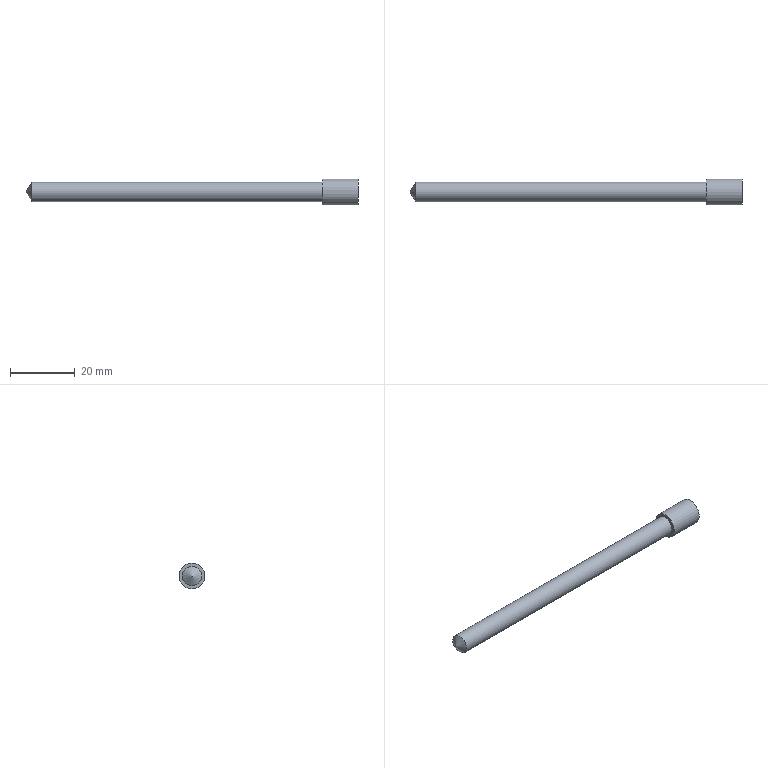Part | NX | features solid 2 | 1 solid | 5 faces | box 102.803 x 8 x 8 mm | volume 3115 mm3 | cylinder 2 | plane 2 | cone 1 | commonest cylinder face diameters 6 x1 8 x1
STEP:
#1=CARTESIAN_POINT('',(44.,-65.,-49.));
#2=VERTEX_POINT('',#1);
#3=CARTESIAN_POINT('',(44.,-65.,-52.));
#4=DIRECTION('',(-1.,0.,0.));
#5=DIRECTION('',(0.,0.,1.));
#6=AXIS2_PLACEMENT_3D('',#3,#4,#5);
#7=CIRCLE('',#6,3.);
#8=EDGE_CURVE('',#2,#2,#7,.F.);
#9=ORIENTED_EDGE('',*,*,#8,.F.);
#10=EDGE_LOOP('',(#9));
#11=FACE_BOUND('',#10,.T.);
#12=CARTESIAN_POINT('',(-46.,-65.,-49.));
#13=VERTEX_POINT('',#12);
#14=CARTESIAN_POINT('',(-46.,-65.,-52.));
#15=DIRECTION('',(1.,0.,0.));
#16=DIRECTION('',(0.,0.,1.));
#17=AXIS2_PLACEMENT_3D('',#14,#15,#16);
#18=CIRCLE('',#17,3.);
#19=EDGE_CURVE('',#13,#13,#18,.T.);
#20=ORIENTED_EDGE('',*,*,#19,.T.);
#21=EDGE_LOOP('',(#20));
#22=FACE_BOUND('',#21,.T.);
#23=CARTESIAN_POINT('',(55.,-65.,-52.));
#24=DIRECTION('',(-1.,0.,0.));
#25=DIRECTION('',(0.,0.,1.));
#26=AXIS2_PLACEMENT_3D('',#23,#24,#25);
#27=CYLINDRICAL_SURFACE('',#26,3.);
#28=ADVANCED_FACE('',(#11,#22),#27,.T.);
#29=ORIENTED_EDGE('',*,*,#19,.F.);
#30=EDGE_LOOP('',(#29));
#31=FACE_BOUND('',#30,.T.);
#32=CARTESIAN_POINT('',(-47.803,-65.,-52.));
#33=VERTEX_POINT('',#32);
#34=VERTEX_LOOP('',#33);
#35=FACE_BOUND('',#34,.T.);
#36=CARTESIAN_POINT('',(-47.803,-65.,-52.));
#37=DIRECTION('',(1.,0.,0.));
#38=DIRECTION('',(0.,0.,1.));
#39=AXIS2_PLACEMENT_3D('',#36,#37,#38);
#40=CONICAL_SURFACE('',#39,0.,1.03);
#41=ADVANCED_FACE('',(#31,#35),#40,.T.);
#42=ORIENTED_EDGE('',*,*,#8,.T.);
#43=EDGE_LOOP('',(#42));
#44=FACE_BOUND('',#43,.T.);
#45=CARTESIAN_POINT('',(44.,-65.,-48.));
#46=VERTEX_POINT('',#45);
#47=CARTESIAN_POINT('',(44.,-65.,-52.));
#48=DIRECTION('',(1.,0.,0.));
#49=DIRECTION('',(0.,0.,1.));
#50=AXIS2_PLACEMENT_3D('',#47,#48,#49);
#51=CIRCLE('',#50,4.);
#52=EDGE_CURVE('',#46,#46,#51,.T.);
#53=ORIENTED_EDGE('',*,*,#52,.F.);
#54=EDGE_LOOP('',(#53));
#55=FACE_BOUND('',#54,.T.);
#56=CARTESIAN_POINT('',(44.,-65.,-52.));
#57=DIRECTION('',(-1.,0.,0.));
#58=DIRECTION('',(0.,0.,1.));
#59=AXIS2_PLACEMENT_3D('',#56,#57,#58);
#60=PLANE('',#59);
#61=ADVANCED_FACE('',(#44,#55),#60,.T.);
#62=ORIENTED_EDGE('',*,*,#52,.T.);
#63=EDGE_LOOP('',(#62));
#64=FACE_BOUND('',#63,.T.);
#65=CARTESIAN_POINT('',(55.,-65.,-48.));
#66=VERTEX_POINT('',#65);
#67=CARTESIAN_POINT('',(55.,-65.,-52.));
#68=DIRECTION('',(-1.,0.,0.));
#69=DIRECTION('',(0.,0.,1.));
#70=AXIS2_PLACEMENT_3D('',#67,#68,#69);
#71=CIRCLE('',#70,4.);
#72=EDGE_CURVE('',#66,#66,#71,.T.);
#73=ORIENTED_EDGE('',*,*,#72,.T.);
#74=EDGE_LOOP('',(#73));
#75=FACE_BOUND('',#74,.T.);
#76=CARTESIAN_POINT('',(55.,-65.,-52.));
#77=DIRECTION('',(-1.,0.,0.));
#78=DIRECTION('',(0.,0.,1.));
#79=AXIS2_PLACEMENT_3D('',#76,#77,#78);
#80=CYLINDRICAL_SURFACE('',#79,4.);
#81=ADVANCED_FACE('',(#64,#75),#80,.T.);
#82=ORIENTED_EDGE('',*,*,#72,.F.);
#83=EDGE_LOOP('',(#82));
#84=FACE_BOUND('',#83,.T.);
#85=CARTESIAN_POINT('',(55.,-65.,-52.));
#86=DIRECTION('',(1.,0.,0.));
#87=DIRECTION('',(0.,0.,-1.));
#88=AXIS2_PLACEMENT_3D('',#85,#86,#87);
#89=PLANE('',#88);
#90=ADVANCED_FACE('',(#84),#89,.T.);
#91=CLOSED_SHELL('',(#28,#41,#61,#81,#90));
#92=MANIFOLD_SOLID_BREP('',#91);
#93=(LENGTH_UNIT()NAMED_UNIT(*)SI_UNIT(.MILLI.,.METRE.));
#94=UNCERTAINTY_MEASURE_WITH_UNIT(LENGTH_MEASURE(0.00001),#93,'','');
#95=(NAMED_UNIT(*)PLANE_ANGLE_UNIT()SI_UNIT($,.RADIAN.));
#96=(NAMED_UNIT(*)SI_UNIT($,.STERADIAN.)SOLID_ANGLE_UNIT());
#97=(GEOMETRIC_REPRESENTATION_CONTEXT(3)GLOBAL_UNCERTAINTY_ASSIGNED_CONTEXT((#94))GLOBAL_UNIT_ASSIGNED_CONTEXT((#93,#95,#96))REPRESENTATION_CONTEXT('',''));
#98=ADVANCED_BREP_SHAPE_REPRESENTATION('',(#92),#97);